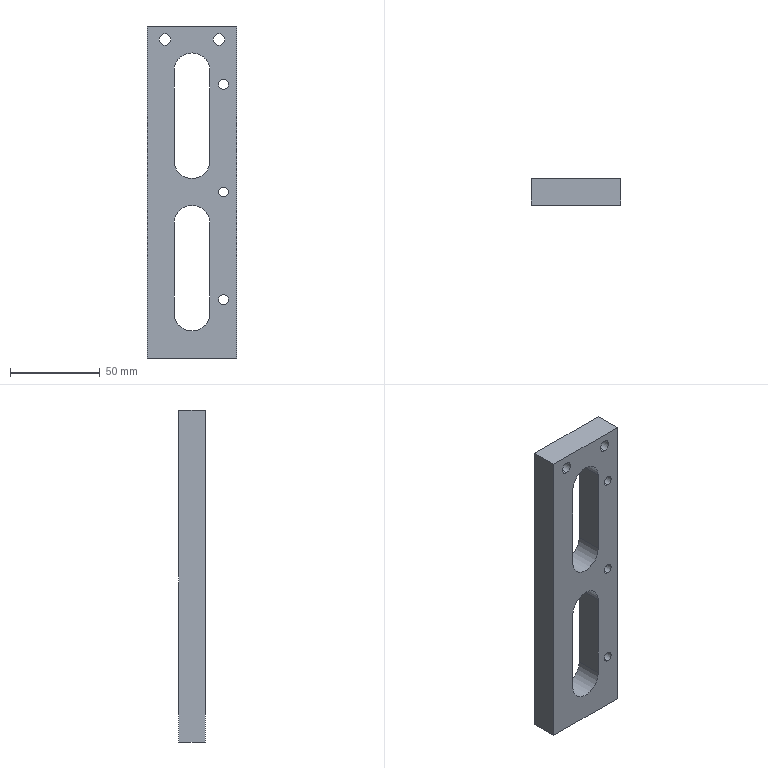Part | STEP file | A14-020 | 1 solid | 49 faces | box 50 x 15 x 185 mm | volume 94203 mm3 | cylinder 30 | plane 15 | cone 4 | commonest cylinder face diameters 5.5 x6 9 x6 20 x6 5 x4 6.5 x4 11 x4